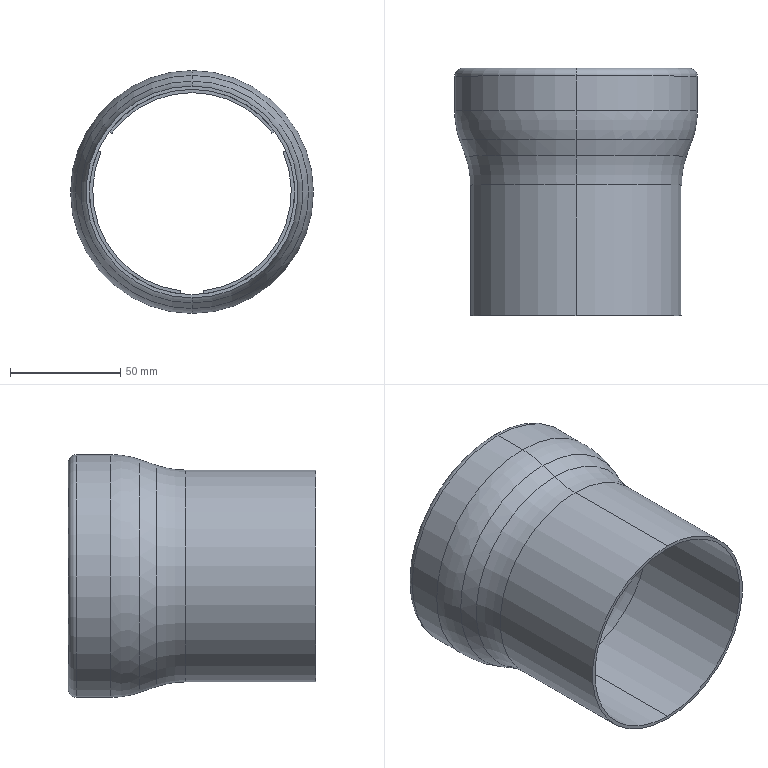Part | SolidWorks | features CirPattern 1, ICE 1, Revolution 1 | 1 solid | 51 faces | box 110 x 112 x 110 mm | volume 57636 mm3 | torus 18 | plane 15 | cylinder 14 | cone 4 | commonest cylinder face diameters 93 x5 90 x3 96 x2 107 x2 110 x2